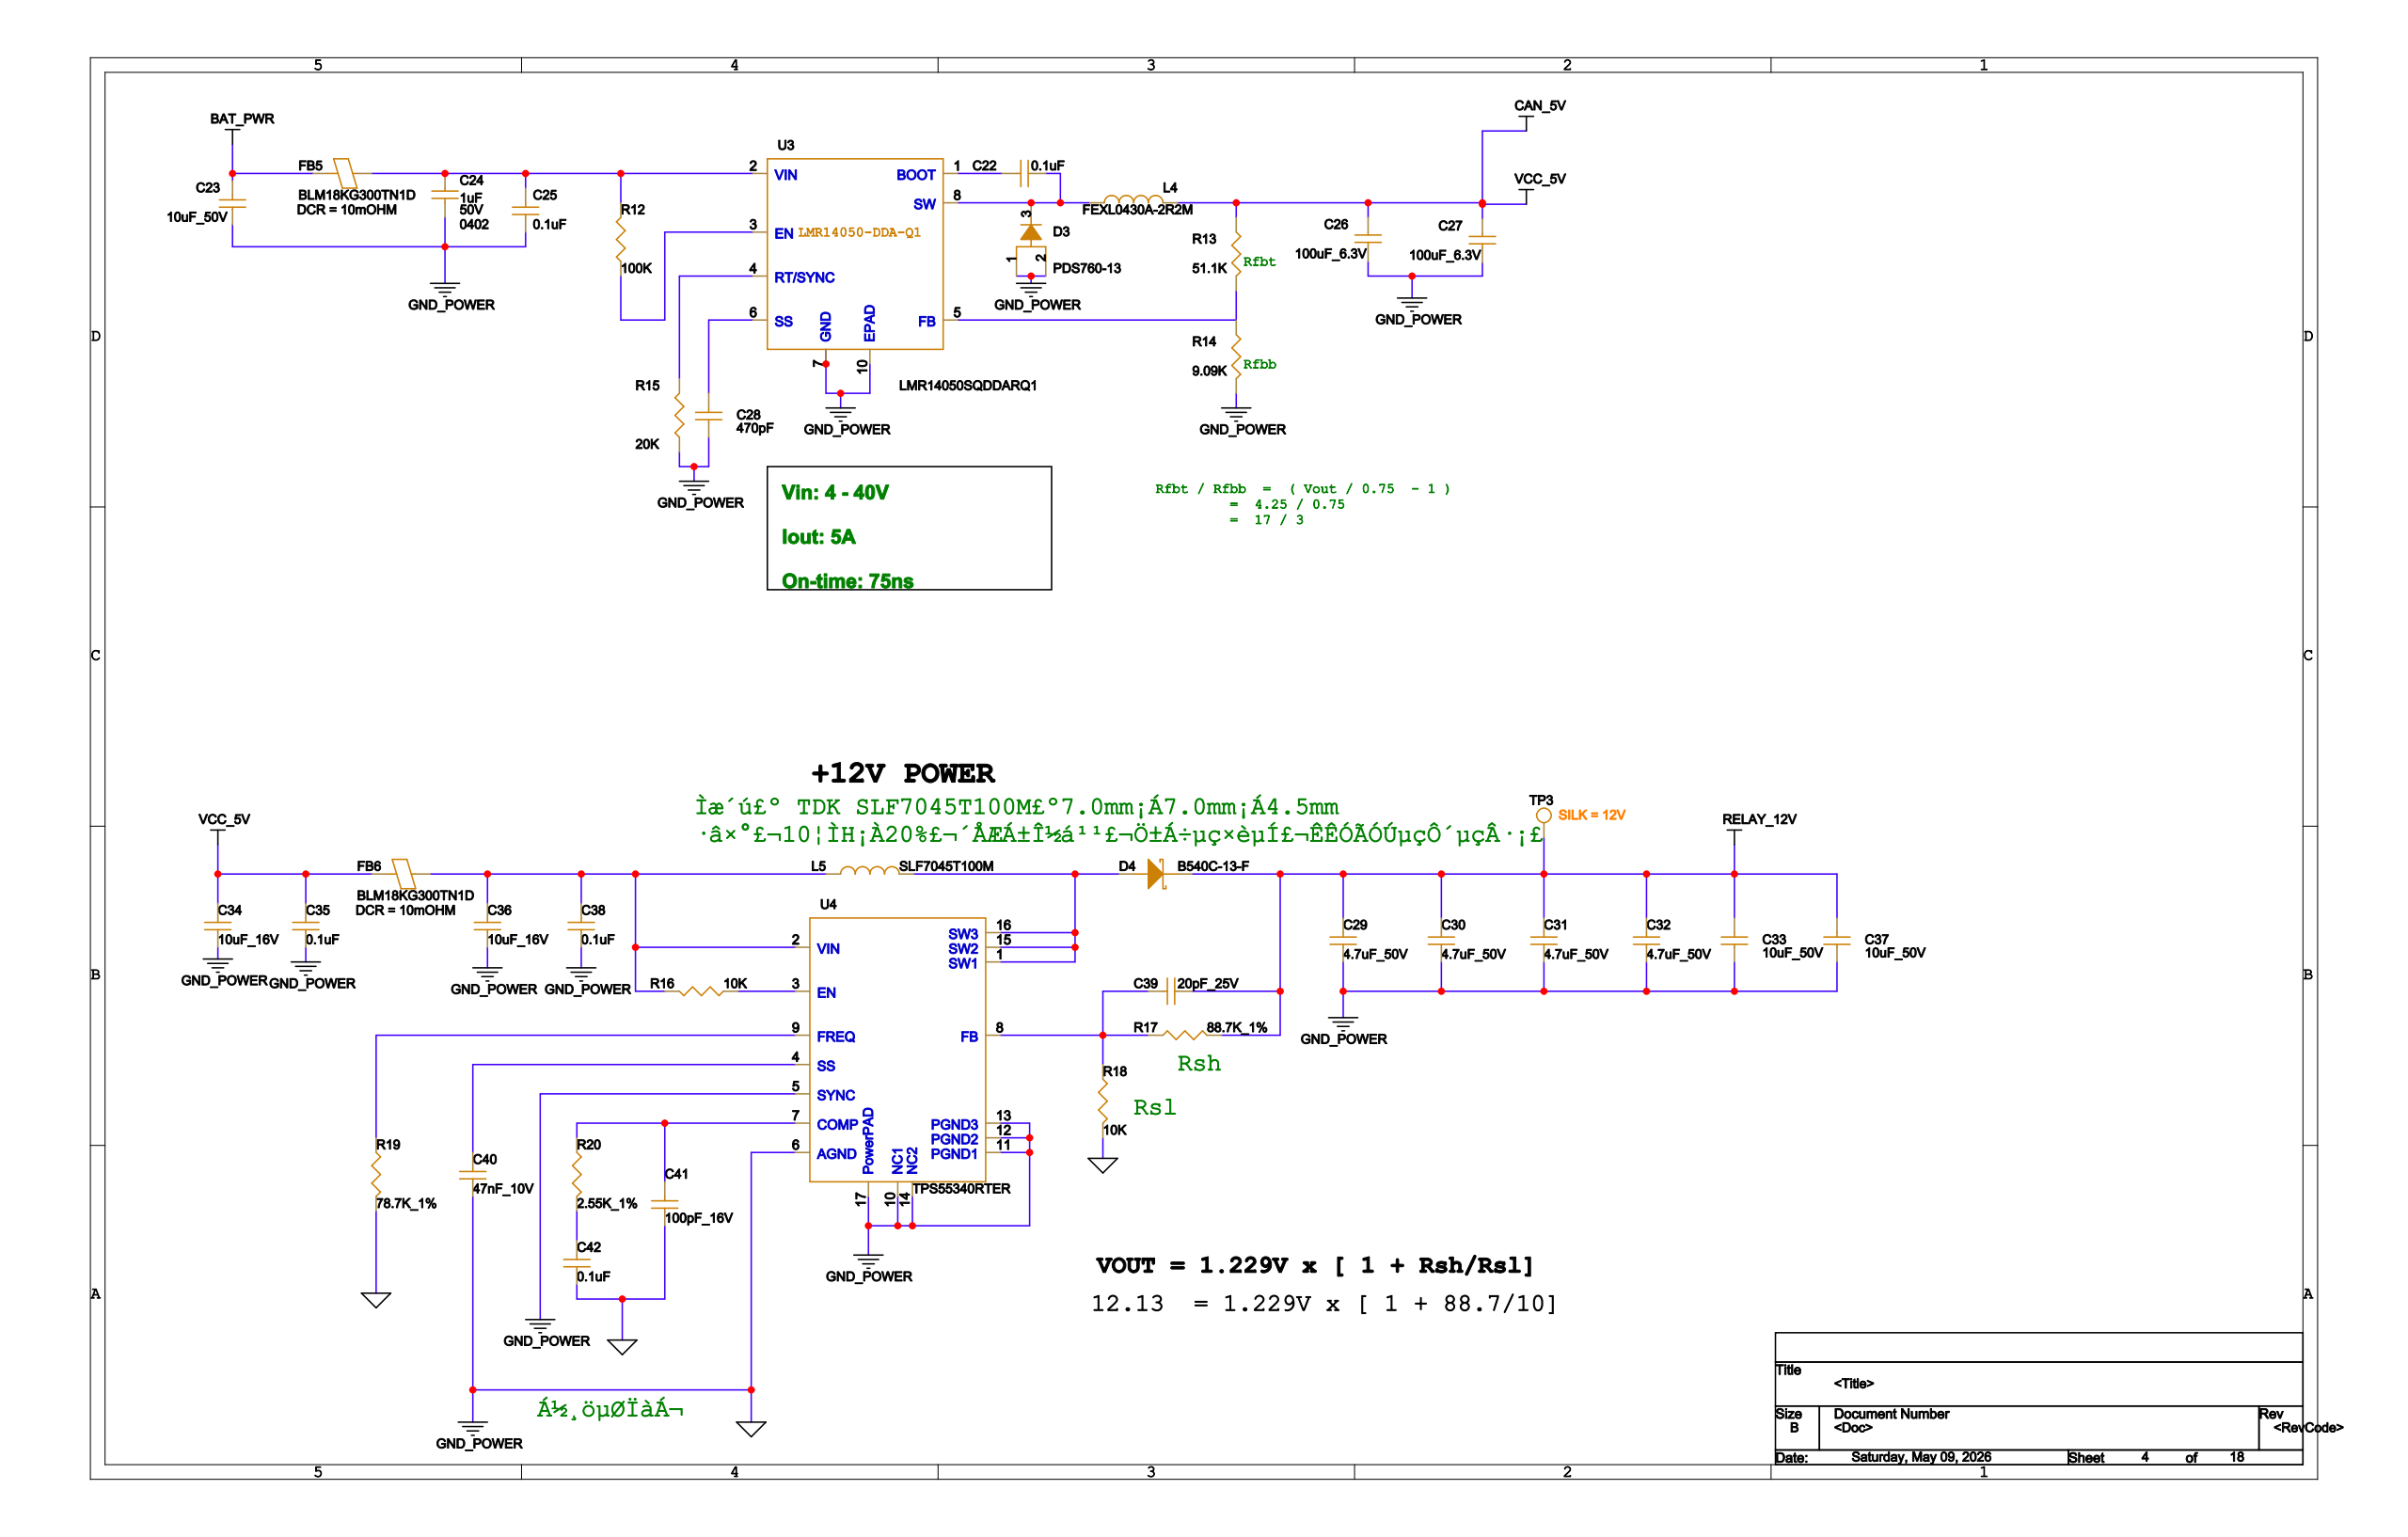Circuit board | Cadence Allegro | 330 parts | 215 nets | one sheet of the schematic
Parts on this sheet (reference | value | footprint):
C22 | 0.1uF | 0402
C23 | 10uF_50V | 1206
C24 | 1uF | 0402
C25 | 0.1uF | 0402
C26 | 100uF_6.3V | 1206
C27 | 100uF_6.3V | 1206
C28 | 470pF | 0402
C29 | 4.7uF_50V | 1210
C30 | 4.7uF_50V | 1210
C31 | 4.7uF_50V | 1210
C32 | 4.7uF_50V | 1210
C33 | 10uF_50V | 1206
C34 | 10uF_16V | 0603
C35 | 0.1uF | 0402
C36 | 10uF_16V | 0603
C37 | 10uF_50V | 1206
C38 | 0.1uF | 0402
C39 | 20pF_25V | 0402
C40 | 47nF_10V | 0402
C41 | 100pF_16V | 0402
C42 | 0.1uF | 0402
D3 | PDS760-13 | PDS760
D4 | B540C-13-F | SMC
FB5 | BLM18KG300TN1D | 0603
FB6 | BLM18KG300TN1D | 0603
L4 | FEXL0430A-2R2M | L_41X41_H210_BOURNS
L5 | SLF7045T100M | SMD_7X7
R12 | 100K | 0402
R13 | 51.1K | 0402
R14 | 9.09K | 0402
R15 | 20K | 0402
R16 | 10K | 0402
R17 | 88.7K_1% | 0402
R18 | 10K | 0402
R19 | 78.7K_1% | 0402
R20 | 2.55K_1% | 0402
TP3 | TP | S0400CI
U3 | LMR14050SQDDARQ1 | SOP8P_60_PAD29X21_127_H170
U4 | TPS55340RTER | WQFN16-3X3
Nets of these parts (net: part-pin ...):
BAT_GND: C23-1 C24-2 C25-1 C26-2 C27-2 C28-1 C29-1 C30-1 C31-1 C32-1 C33-1 C34-1 C35-1 C36-1 C37-1 C38-1 C40-1 C41-1 C42-1 D3-1 D3-2 R14-2 R15-1 R18-2 R19-2 U3-7 U3-10 U4-5 U4-6 U4-10 U4-11 U4-12 U4-13 U4-14 U4-17
N16894931: C24-1 C25-2 FB5-1 R12-2 U3-2
CAN_5V: C26-1 C27-1 C34-2 C35-2 FB6-2 L4-2 R13-1
BAT_PWR: C23-2 FB5-2
N16895535: C41-2 R20-1 U4-7
N16895474: R16-1 U4-3
N16895476: C39-2 R17-1 R18-1 U4-8
N16895507: R19-1 U4-9
N16895519: C40-2 U4-4
N16895329: D4-2 L5-2 U4-1 U4-15 U4-16
N16895322: C36-2 C38-2 FB6-1 L5-1 R16-2 U4-2
RELAY_12V: C29-2 C30-2 C31-2 C32-2 C33-2 C37-2 C39-1 D4-1 R17-2 TP3-1
N16895056: R12-1 U3-3
N16895096: R15-2 U3-4
N16895605: C42-2 R20-2
N16894945: C22-1 D3-3 L4-1 U3-8
N16895125: C28-2 U3-6
N16895118: R13-2 R14-1 U3-5
N16894943: C22-2 U3-1